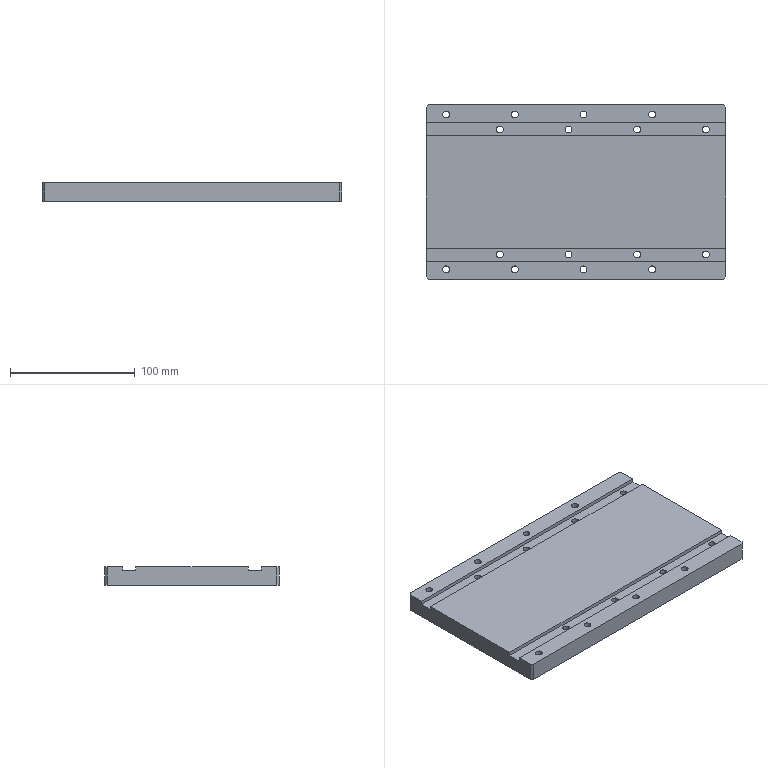Part | STEP file | 08-06 conveyor base plate | 1 solid | 74 faces | box 240 x 140 x 15 mm | volume 481130 mm3 | cylinder 48 | plane 26 | commonest cylinder face diameters 5.5 x32 10 x16